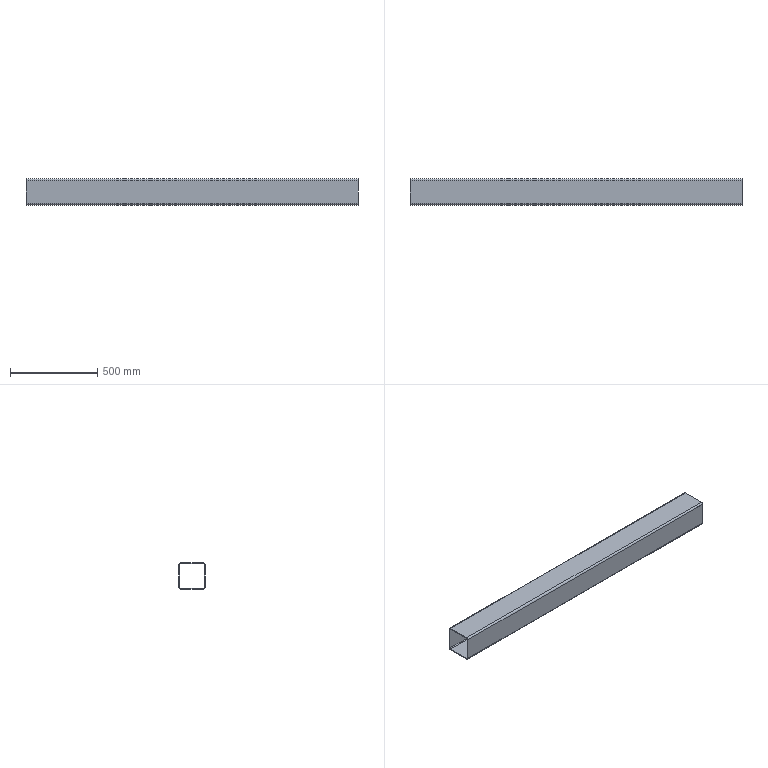Part | SolidWorks | features WeldMemberFeat 1, WeldmentFeature 1 | 1 solid | 18 faces | box 1900 x 150 x 150 mm | volume 5387677 mm3 | plane 10 | cylinder 8 | commonest cylinder face diameters 10 x4 20 x4
STEP:
#1=CARTESIAN_POINT('',(-950.,75.,65.));
#2=VERTEX_POINT('',#1);
#3=CARTESIAN_POINT('',(-950.,65.,75.));
#4=VERTEX_POINT('',#3);
#5=CARTESIAN_POINT('',(-950.,65.,65.));
#6=DIRECTION('',(1.,0.,0.));
#7=DIRECTION('',(0.,1.,0.));
#8=AXIS2_PLACEMENT_3D('',#5,#6,#7);
#9=CIRCLE('',#8,10.);
#10=EDGE_CURVE('',#2,#4,#9,.T.);
#11=ORIENTED_EDGE('',*,*,#10,.T.);
#12=CARTESIAN_POINT('',(950.,65.,75.));
#13=VERTEX_POINT('',#12);
#14=CARTESIAN_POINT('',(950.,65.,75.));
#15=DIRECTION('',(-1.,0.,0.));
#16=VECTOR('',#15,1000.);
#17=LINE('',#14,#16);
#18=EDGE_CURVE('',#13,#4,#17,.T.);
#19=ORIENTED_EDGE('',*,*,#18,.F.);
#20=CARTESIAN_POINT('',(950.,75.,65.));
#21=VERTEX_POINT('',#20);
#22=CARTESIAN_POINT('',(950.,65.,65.));
#23=DIRECTION('',(1.,0.,0.));
#24=DIRECTION('',(0.,1.,0.));
#25=AXIS2_PLACEMENT_3D('',#22,#23,#24);
#26=CIRCLE('',#25,10.);
#27=EDGE_CURVE('',#21,#13,#26,.T.);
#28=ORIENTED_EDGE('',*,*,#27,.F.);
#29=CARTESIAN_POINT('',(950.,75.,65.));
#30=DIRECTION('',(-1.,0.,0.));
#31=VECTOR('',#30,1000.);
#32=LINE('',#29,#31);
#33=EDGE_CURVE('',#21,#2,#32,.T.);
#34=ORIENTED_EDGE('',*,*,#33,.T.);
#35=EDGE_LOOP('',(#11,#19,#28,#34));
#36=FACE_OUTER_BOUND('',#35,.T.);
#37=CARTESIAN_POINT('',(950.,65.,65.));
#38=DIRECTION('',(-1.,0.,0.));
#39=DIRECTION('',(0.,-1.,0.));
#40=AXIS2_PLACEMENT_3D('',#37,#38,#39);
#41=CYLINDRICAL_SURFACE('',#40,10.);
#42=ADVANCED_FACE('',(#36),#41,.T.);
#43=CARTESIAN_POINT('',(-950.,-65.,75.));
#44=VERTEX_POINT('',#43);
#45=CARTESIAN_POINT('',(-950.,65.,75.));
#46=DIRECTION('',(0.,-1.,0.));
#47=VECTOR('',#46,1000.);
#48=LINE('',#45,#47);
#49=EDGE_CURVE('',#4,#44,#48,.T.);
#50=ORIENTED_EDGE('',*,*,#49,.T.);
#51=CARTESIAN_POINT('',(950.,-65.,75.));
#52=VERTEX_POINT('',#51);
#53=CARTESIAN_POINT('',(950.,-65.,75.));
#54=DIRECTION('',(-1.,0.,0.));
#55=VECTOR('',#54,1000.);
#56=LINE('',#53,#55);
#57=EDGE_CURVE('',#52,#44,#56,.T.);
#58=ORIENTED_EDGE('',*,*,#57,.F.);
#59=CARTESIAN_POINT('',(950.,65.,75.));
#60=DIRECTION('',(0.,-1.,0.));
#61=VECTOR('',#60,1000.);
#62=LINE('',#59,#61);
#63=EDGE_CURVE('',#13,#52,#62,.T.);
#64=ORIENTED_EDGE('',*,*,#63,.F.);
#65=ORIENTED_EDGE('',*,*,#18,.T.);
#66=EDGE_LOOP('',(#50,#58,#64,#65));
#67=FACE_OUTER_BOUND('',#66,.T.);
#68=CARTESIAN_POINT('',(950.,65.,75.));
#69=DIRECTION('',(0.,0.,-1.));
#70=DIRECTION('',(-1.,0.,0.));
#71=AXIS2_PLACEMENT_3D('',#68,#69,#70);
#72=PLANE('',#71);
#73=ADVANCED_FACE('',(#67),#72,.F.);
#74=CARTESIAN_POINT('',(-950.,-75.,65.));
#75=VERTEX_POINT('',#74);
#76=CARTESIAN_POINT('',(-950.,-65.,65.));
#77=DIRECTION('',(1.,0.,0.));
#78=DIRECTION('',(0.,1.,0.));
#79=AXIS2_PLACEMENT_3D('',#76,#77,#78);
#80=CIRCLE('',#79,10.);
#81=EDGE_CURVE('',#44,#75,#80,.T.);
#82=ORIENTED_EDGE('',*,*,#81,.T.);
#83=CARTESIAN_POINT('',(950.,-75.,65.));
#84=VERTEX_POINT('',#83);
#85=CARTESIAN_POINT('',(950.,-75.,65.));
#86=DIRECTION('',(-1.,0.,0.));
#87=VECTOR('',#86,1000.);
#88=LINE('',#85,#87);
#89=EDGE_CURVE('',#84,#75,#88,.T.);
#90=ORIENTED_EDGE('',*,*,#89,.F.);
#91=CARTESIAN_POINT('',(950.,-65.,65.));
#92=DIRECTION('',(1.,0.,0.));
#93=DIRECTION('',(0.,1.,0.));
#94=AXIS2_PLACEMENT_3D('',#91,#92,#93);
#95=CIRCLE('',#94,10.);
#96=EDGE_CURVE('',#52,#84,#95,.T.);
#97=ORIENTED_EDGE('',*,*,#96,.F.);
#98=ORIENTED_EDGE('',*,*,#57,.T.);
#99=EDGE_LOOP('',(#82,#90,#97,#98));
#100=FACE_OUTER_BOUND('',#99,.T.);
#101=CARTESIAN_POINT('',(950.,-65.,65.));
#102=DIRECTION('',(-1.,0.,0.));
#103=DIRECTION('',(0.,-1.,0.));
#104=AXIS2_PLACEMENT_3D('',#101,#102,#103);
#105=CYLINDRICAL_SURFACE('',#104,10.);
#106=ADVANCED_FACE('',(#100),#105,.T.);
#107=CARTESIAN_POINT('',(-950.,-75.,-65.));
#108=VERTEX_POINT('',#107);
#109=CARTESIAN_POINT('',(-950.,-75.,-65.));
#110=DIRECTION('',(0.,0.,-1.));
#111=VECTOR('',#110,1000.);
#112=LINE('',#109,#111);
#113=EDGE_CURVE('',#75,#108,#112,.T.);
#114=ORIENTED_EDGE('',*,*,#113,.T.);
#115=CARTESIAN_POINT('',(950.,-75.,-65.));
#116=VERTEX_POINT('',#115);
#117=CARTESIAN_POINT('',(950.,-75.,-65.));
#118=DIRECTION('',(-1.,0.,0.));
#119=VECTOR('',#118,1000.);
#120=LINE('',#117,#119);
#121=EDGE_CURVE('',#116,#108,#120,.T.);
#122=ORIENTED_EDGE('',*,*,#121,.F.);
#123=CARTESIAN_POINT('',(950.,-75.,-65.));
#124=DIRECTION('',(0.,0.,-1.));
#125=VECTOR('',#124,1000.);
#126=LINE('',#123,#125);
#127=EDGE_CURVE('',#84,#116,#126,.T.);
#128=ORIENTED_EDGE('',*,*,#127,.F.);
#129=ORIENTED_EDGE('',*,*,#89,.T.);
#130=EDGE_LOOP('',(#114,#122,#128,#129));
#131=FACE_OUTER_BOUND('',#130,.T.);
#132=CARTESIAN_POINT('',(950.,-75.,-65.));
#133=DIRECTION('',(0.,1.,0.));
#134=DIRECTION('',(-1.,0.,0.));
#135=AXIS2_PLACEMENT_3D('',#132,#133,#134);
#136=PLANE('',#135);
#137=ADVANCED_FACE('',(#131),#136,.F.);
#138=CARTESIAN_POINT('',(-950.,-65.,-75.));
#139=VERTEX_POINT('',#138);
#140=CARTESIAN_POINT('',(-950.,-65.,-65.));
#141=DIRECTION('',(1.,0.,0.));
#142=DIRECTION('',(0.,1.,0.));
#143=AXIS2_PLACEMENT_3D('',#140,#141,#142);
#144=CIRCLE('',#143,10.);
#145=EDGE_CURVE('',#108,#139,#144,.T.);
#146=ORIENTED_EDGE('',*,*,#145,.T.);
#147=CARTESIAN_POINT('',(950.,-65.,-75.));
#148=VERTEX_POINT('',#147);
#149=CARTESIAN_POINT('',(950.,-65.,-75.));
#150=DIRECTION('',(-1.,0.,0.));
#151=VECTOR('',#150,1000.);
#152=LINE('',#149,#151);
#153=EDGE_CURVE('',#148,#139,#152,.T.);
#154=ORIENTED_EDGE('',*,*,#153,.F.);
#155=CARTESIAN_POINT('',(950.,-65.,-65.));
#156=DIRECTION('',(1.,0.,0.));
#157=DIRECTION('',(0.,1.,0.));
#158=AXIS2_PLACEMENT_3D('',#155,#156,#157);
#159=CIRCLE('',#158,10.);
#160=EDGE_CURVE('',#116,#148,#159,.T.);
#161=ORIENTED_EDGE('',*,*,#160,.F.);
#162=ORIENTED_EDGE('',*,*,#121,.T.);
#163=EDGE_LOOP('',(#146,#154,#161,#162));
#164=FACE_OUTER_BOUND('',#163,.T.);
#165=CARTESIAN_POINT('',(950.,-65.,-65.));
#166=DIRECTION('',(-1.,0.,0.));
#167=DIRECTION('',(0.,-1.,0.));
#168=AXIS2_PLACEMENT_3D('',#165,#166,#167);
#169=CYLINDRICAL_SURFACE('',#168,10.);
#170=ADVANCED_FACE('',(#164),#169,.T.);
#171=CARTESIAN_POINT('',(-950.,65.,-75.));
#172=VERTEX_POINT('',#171);
#173=CARTESIAN_POINT('',(-950.,-65.,-75.));
#174=DIRECTION('',(0.,1.,0.));
#175=VECTOR('',#174,1000.);
#176=LINE('',#173,#175);
#177=EDGE_CURVE('',#139,#172,#176,.T.);
#178=ORIENTED_EDGE('',*,*,#177,.T.);
#179=CARTESIAN_POINT('',(950.,65.,-75.));
#180=VERTEX_POINT('',#179);
#181=CARTESIAN_POINT('',(950.,65.,-75.));
#182=DIRECTION('',(-1.,0.,0.));
#183=VECTOR('',#182,1000.);
#184=LINE('',#181,#183);
#185=EDGE_CURVE('',#180,#172,#184,.T.);
#186=ORIENTED_EDGE('',*,*,#185,.F.);
#187=CARTESIAN_POINT('',(950.,-65.,-75.));
#188=DIRECTION('',(0.,1.,0.));
#189=VECTOR('',#188,1000.);
#190=LINE('',#187,#189);
#191=EDGE_CURVE('',#148,#180,#190,.T.);
#192=ORIENTED_EDGE('',*,*,#191,.F.);
#193=ORIENTED_EDGE('',*,*,#153,.T.);
#194=EDGE_LOOP('',(#178,#186,#192,#193));
#195=FACE_OUTER_BOUND('',#194,.T.);
#196=CARTESIAN_POINT('',(950.,-65.,-75.));
#197=DIRECTION('',(0.,0.,1.));
#198=DIRECTION('',(1.,0.,0.));
#199=AXIS2_PLACEMENT_3D('',#196,#197,#198);
#200=PLANE('',#199);
#201=ADVANCED_FACE('',(#195),#200,.F.);
#202=CARTESIAN_POINT('',(-950.,75.,-65.));
#203=VERTEX_POINT('',#202);
#204=CARTESIAN_POINT('',(-950.,65.,-65.));
#205=DIRECTION('',(1.,0.,0.));
#206=DIRECTION('',(0.,1.,0.));
#207=AXIS2_PLACEMENT_3D('',#204,#205,#206);
#208=CIRCLE('',#207,10.);
#209=EDGE_CURVE('',#172,#203,#208,.T.);
#210=ORIENTED_EDGE('',*,*,#209,.T.);
#211=CARTESIAN_POINT('',(950.,75.,-65.));
#212=VERTEX_POINT('',#211);
#213=CARTESIAN_POINT('',(950.,75.,-65.));
#214=DIRECTION('',(-1.,0.,0.));
#215=VECTOR('',#214,1000.);
#216=LINE('',#213,#215);
#217=EDGE_CURVE('',#212,#203,#216,.T.);
#218=ORIENTED_EDGE('',*,*,#217,.F.);
#219=CARTESIAN_POINT('',(950.,65.,-65.));
#220=DIRECTION('',(1.,0.,0.));
#221=DIRECTION('',(0.,1.,0.));
#222=AXIS2_PLACEMENT_3D('',#219,#220,#221);
#223=CIRCLE('',#222,10.);
#224=EDGE_CURVE('',#180,#212,#223,.T.);
#225=ORIENTED_EDGE('',*,*,#224,.F.);
#226=ORIENTED_EDGE('',*,*,#185,.T.);
#227=EDGE_LOOP('',(#210,#218,#225,#226));
#228=FACE_OUTER_BOUND('',#227,.T.);
#229=CARTESIAN_POINT('',(950.,65.,-65.));
#230=DIRECTION('',(-1.,0.,0.));
#231=DIRECTION('',(0.,-1.,0.));
#232=AXIS2_PLACEMENT_3D('',#229,#230,#231);
#233=CYLINDRICAL_SURFACE('',#232,10.);
#234=ADVANCED_FACE('',(#228),#233,.T.);
#235=CARTESIAN_POINT('',(-950.,-65.,70.));
#236=VERTEX_POINT('',#235);
#237=CARTESIAN_POINT('',(-950.,-70.,65.));
#238=VERTEX_POINT('',#237);
#239=CARTESIAN_POINT('',(-950.,-65.,65.));
#240=DIRECTION('',(1.,0.,0.));
#241=DIRECTION('',(0.,1.,0.));
#242=AXIS2_PLACEMENT_3D('',#239,#240,#241);
#243=CIRCLE('',#242,5.);
#244=EDGE_CURVE('',#236,#238,#243,.T.);
#245=ORIENTED_EDGE('',*,*,#244,.F.);
#246=CARTESIAN_POINT('',(950.,-65.,70.));
#247=VERTEX_POINT('',#246);
#248=CARTESIAN_POINT('',(950.,-65.,70.));
#249=DIRECTION('',(-1.,0.,0.));
#250=VECTOR('',#249,1000.);
#251=LINE('',#248,#250);
#252=EDGE_CURVE('',#247,#236,#251,.T.);
#253=ORIENTED_EDGE('',*,*,#252,.F.);
#254=CARTESIAN_POINT('',(950.,-70.,65.));
#255=VERTEX_POINT('',#254);
#256=CARTESIAN_POINT('',(950.,-65.,65.));
#257=DIRECTION('',(1.,0.,0.));
#258=DIRECTION('',(0.,1.,0.));
#259=AXIS2_PLACEMENT_3D('',#256,#257,#258);
#260=CIRCLE('',#259,5.);
#261=EDGE_CURVE('',#247,#255,#260,.T.);
#262=ORIENTED_EDGE('',*,*,#261,.T.);
#263=CARTESIAN_POINT('',(950.,-70.,65.));
#264=DIRECTION('',(-1.,0.,0.));
#265=VECTOR('',#264,1000.);
#266=LINE('',#263,#265);
#267=EDGE_CURVE('',#255,#238,#266,.T.);
#268=ORIENTED_EDGE('',*,*,#267,.T.);
#269=EDGE_LOOP('',(#245,#253,#262,#268));
#270=FACE_OUTER_BOUND('',#269,.T.);
#271=CARTESIAN_POINT('',(950.,-65.,65.));
#272=DIRECTION('',(-1.,0.,0.));
#273=DIRECTION('',(0.,-1.,0.));
#274=AXIS2_PLACEMENT_3D('',#271,#272,#273);
#275=CYLINDRICAL_SURFACE('',#274,5.);
#276=ADVANCED_FACE('',(#270),#275,.F.);
#277=CARTESIAN_POINT('',(-950.,65.,70.));
#278=VERTEX_POINT('',#277);
#279=CARTESIAN_POINT('',(-950.,65.,70.));
#280=DIRECTION('',(0.,-1.,0.));
#281=VECTOR('',#280,1000.);
#282=LINE('',#279,#281);
#283=EDGE_CURVE('',#278,#236,#282,.T.);
#284=ORIENTED_EDGE('',*,*,#283,.F.);
#285=CARTESIAN_POINT('',(950.,65.,70.));
#286=VERTEX_POINT('',#285);
#287=CARTESIAN_POINT('',(950.,65.,70.));
#288=DIRECTION('',(-1.,0.,0.));
#289=VECTOR('',#288,1000.);
#290=LINE('',#287,#289);
#291=EDGE_CURVE('',#286,#278,#290,.T.);
#292=ORIENTED_EDGE('',*,*,#291,.F.);
#293=CARTESIAN_POINT('',(950.,65.,70.));
#294=DIRECTION('',(0.,-1.,0.));
#295=VECTOR('',#294,1000.);
#296=LINE('',#293,#295);
#297=EDGE_CURVE('',#286,#247,#296,.T.);
#298=ORIENTED_EDGE('',*,*,#297,.T.);
#299=ORIENTED_EDGE('',*,*,#252,.T.);
#300=EDGE_LOOP('',(#284,#292,#298,#299));
#301=FACE_OUTER_BOUND('',#300,.T.);
#302=CARTESIAN_POINT('',(950.,65.,70.));
#303=DIRECTION('',(0.,0.,-1.));
#304=DIRECTION('',(-1.,0.,0.));
#305=AXIS2_PLACEMENT_3D('',#302,#303,#304);
#306=PLANE('',#305);
#307=ADVANCED_FACE('',(#301),#306,.T.);
#308=CARTESIAN_POINT('',(-950.,70.,65.));
#309=VERTEX_POINT('',#308);
#310=CARTESIAN_POINT('',(-950.,65.,65.));
#311=DIRECTION('',(1.,0.,0.));
#312=DIRECTION('',(0.,1.,0.));
#313=AXIS2_PLACEMENT_3D('',#310,#311,#312);
#314=CIRCLE('',#313,5.);
#315=EDGE_CURVE('',#309,#278,#314,.T.);
#316=ORIENTED_EDGE('',*,*,#315,.F.);
#317=CARTESIAN_POINT('',(950.,70.,65.));
#318=VERTEX_POINT('',#317);
#319=CARTESIAN_POINT('',(950.,70.,65.));
#320=DIRECTION('',(-1.,0.,0.));
#321=VECTOR('',#320,1000.);
#322=LINE('',#319,#321);
#323=EDGE_CURVE('',#318,#309,#322,.T.);
#324=ORIENTED_EDGE('',*,*,#323,.F.);
#325=CARTESIAN_POINT('',(950.,65.,65.));
#326=DIRECTION('',(1.,0.,0.));
#327=DIRECTION('',(0.,1.,0.));
#328=AXIS2_PLACEMENT_3D('',#325,#326,#327);
#329=CIRCLE('',#328,5.);
#330=EDGE_CURVE('',#318,#286,#329,.T.);
#331=ORIENTED_EDGE('',*,*,#330,.T.);
#332=ORIENTED_EDGE('',*,*,#291,.T.);
#333=EDGE_LOOP('',(#316,#324,#331,#332));
#334=FACE_OUTER_BOUND('',#333,.T.);
#335=CARTESIAN_POINT('',(950.,65.,65.));
#336=DIRECTION('',(-1.,0.,0.));
#337=DIRECTION('',(0.,-1.,0.));
#338=AXIS2_PLACEMENT_3D('',#335,#336,#337);
#339=CYLINDRICAL_SURFACE('',#338,5.);
#340=ADVANCED_FACE('',(#334),#339,.F.);
#341=CARTESIAN_POINT('',(-950.,70.,-65.));
#342=VERTEX_POINT('',#341);
#343=CARTESIAN_POINT('',(-950.,70.,65.));
#344=DIRECTION('',(0.,0.,1.));
#345=VECTOR('',#344,1000.);
#346=LINE('',#343,#345);
#347=EDGE_CURVE('',#342,#309,#346,.T.);
#348=ORIENTED_EDGE('',*,*,#347,.F.);
#349=CARTESIAN_POINT('',(950.,70.,-65.));
#350=VERTEX_POINT('',#349);
#351=CARTESIAN_POINT('',(950.,70.,-65.));
#352=DIRECTION('',(-1.,0.,0.));
#353=VECTOR('',#352,1000.);
#354=LINE('',#351,#353);
#355=EDGE_CURVE('',#350,#342,#354,.T.);
#356=ORIENTED_EDGE('',*,*,#355,.F.);
#357=CARTESIAN_POINT('',(950.,70.,65.));
#358=DIRECTION('',(0.,0.,1.));
#359=VECTOR('',#358,1000.);
#360=LINE('',#357,#359);
#361=EDGE_CURVE('',#350,#318,#360,.T.);
#362=ORIENTED_EDGE('',*,*,#361,.T.);
#363=ORIENTED_EDGE('',*,*,#323,.T.);
#364=EDGE_LOOP('',(#348,#356,#362,#363));
#365=FACE_OUTER_BOUND('',#364,.T.);
#366=CARTESIAN_POINT('',(950.,70.,65.));
#367=DIRECTION('',(0.,-1.,0.));
#368=DIRECTION('',(1.,0.,0.));
#369=AXIS2_PLACEMENT_3D('',#366,#367,#368);
#370=PLANE('',#369);
#371=ADVANCED_FACE('',(#365),#370,.T.);
#372=CARTESIAN_POINT('',(-950.,65.,-70.));
#373=VERTEX_POINT('',#372);
#374=CARTESIAN_POINT('',(-950.,65.,-65.));
#375=DIRECTION('',(1.,0.,0.));
#376=DIRECTION('',(0.,1.,0.));
#377=AXIS2_PLACEMENT_3D('',#374,#375,#376);
#378=CIRCLE('',#377,5.);
#379=EDGE_CURVE('',#373,#342,#378,.T.);
#380=ORIENTED_EDGE('',*,*,#379,.F.);
#381=CARTESIAN_POINT('',(950.,65.,-70.));
#382=VERTEX_POINT('',#381);
#383=CARTESIAN_POINT('',(950.,65.,-70.));
#384=DIRECTION('',(-1.,0.,0.));
#385=VECTOR('',#384,1000.);
#386=LINE('',#383,#385);
#387=EDGE_CURVE('',#382,#373,#386,.T.);
#388=ORIENTED_EDGE('',*,*,#387,.F.);
#389=CARTESIAN_POINT('',(950.,65.,-65.));
#390=DIRECTION('',(1.,0.,0.));
#391=DIRECTION('',(0.,1.,0.));
#392=AXIS2_PLACEMENT_3D('',#389,#390,#391);
#393=CIRCLE('',#392,5.);
#394=EDGE_CURVE('',#382,#350,#393,.T.);
#395=ORIENTED_EDGE('',*,*,#394,.T.);
#396=ORIENTED_EDGE('',*,*,#355,.T.);
#397=EDGE_LOOP('',(#380,#388,#395,#396));
#398=FACE_OUTER_BOUND('',#397,.T.);
#399=CARTESIAN_POINT('',(950.,65.,-65.));
#400=DIRECTION('',(-1.,0.,0.));
#401=DIRECTION('',(0.,-1.,0.));
#402=AXIS2_PLACEMENT_3D('',#399,#400,#401);
#403=CYLINDRICAL_SURFACE('',#402,5.);
#404=ADVANCED_FACE('',(#398),#403,.F.);
#405=CARTESIAN_POINT('',(-950.,-65.,-70.));
#406=VERTEX_POINT('',#405);
#407=CARTESIAN_POINT('',(-950.,-65.,-70.));
#408=DIRECTION('',(0.,1.,0.));
#409=VECTOR('',#408,1000.);
#410=LINE('',#407,#409);
#411=EDGE_CURVE('',#406,#373,#410,.T.);
#412=ORIENTED_EDGE('',*,*,#411,.F.);
#413=CARTESIAN_POINT('',(950.,-65.,-70.));
#414=VERTEX_POINT('',#413);
#415=CARTESIAN_POINT('',(950.,-65.,-70.));
#416=DIRECTION('',(-1.,0.,0.));
#417=VECTOR('',#416,1000.);
#418=LINE('',#415,#417);
#419=EDGE_CURVE('',#414,#406,#418,.T.);
#420=ORIENTED_EDGE('',*,*,#419,.F.);
#421=CARTESIAN_POINT('',(950.,-65.,-70.));
#422=DIRECTION('',(0.,1.,0.));
#423=VECTOR('',#422,1000.);
#424=LINE('',#421,#423);
#425=EDGE_CURVE('',#414,#382,#424,.T.);
#426=ORIENTED_EDGE('',*,*,#425,.T.);
#427=ORIENTED_EDGE('',*,*,#387,.T.);
#428=EDGE_LOOP('',(#412,#420,#426,#427));
#429=FACE_OUTER_BOUND('',#428,.T.);
#430=CARTESIAN_POINT('',(950.,-65.,-70.));
#431=DIRECTION('',(0.,0.,1.));
#432=DIRECTION('',(1.,0.,0.));
#433=AXIS2_PLACEMENT_3D('',#430,#431,#432);
#434=PLANE('',#433);
#435=ADVANCED_FACE('',(#429),#434,.T.);
#436=CARTESIAN_POINT('',(-950.,-70.,-65.));
#437=VERTEX_POINT('',#436);
#438=CARTESIAN_POINT('',(-950.,-65.,-65.));
#439=DIRECTION('',(1.,0.,0.));
#440=DIRECTION('',(0.,1.,0.));
#441=AXIS2_PLACEMENT_3D('',#438,#439,#440);
#442=CIRCLE('',#441,5.);
#443=EDGE_CURVE('',#437,#406,#442,.T.);
#444=ORIENTED_EDGE('',*,*,#443,.F.);
#445=CARTESIAN_POINT('',(950.,-70.,-65.));
#446=VERTEX_POINT('',#445);
#447=CARTESIAN_POINT('',(950.,-70.,-65.));
#448=DIRECTION('',(-1.,0.,0.));
#449=VECTOR('',#448,1000.);
#450=LINE('',#447,#449);
#451=EDGE_CURVE('',#446,#437,#450,.T.);
#452=ORIENTED_EDGE('',*,*,#451,.F.);
#453=CARTESIAN_POINT('',(950.,-65.,-65.));
#454=DIRECTION('',(1.,0.,0.));
#455=DIRECTION('',(0.,1.,0.));
#456=AXIS2_PLACEMENT_3D('',#453,#454,#455);
#457=CIRCLE('',#456,5.);
#458=EDGE_CURVE('',#446,#414,#457,.T.);
#459=ORIENTED_EDGE('',*,*,#458,.T.);
#460=ORIENTED_EDGE('',*,*,#419,.T.);
#461=EDGE_LOOP('',(#444,#452,#459,#460));
#462=FACE_OUTER_BOUND('',#461,.T.);
#463=CARTESIAN_POINT('',(950.,-65.,-65.));
#464=DIRECTION('',(-1.,0.,0.));
#465=DIRECTION('',(0.,-1.,0.));
#466=AXIS2_PLACEMENT_3D('',#463,#464,#465);
#467=CYLINDRICAL_SURFACE('',#466,5.);
#468=ADVANCED_FACE('',(#462),#467,.F.);
#469=CARTESIAN_POINT('',(-950.,-70.,-65.));
#470=DIRECTION('',(0.,0.,-1.));
#471=VECTOR('',#470,1000.);
#472=LINE('',#469,#471);
#473=EDGE_CURVE('',#238,#437,#472,.T.);
#474=ORIENTED_EDGE('',*,*,#473,.F.);
#475=ORIENTED_EDGE('',*,*,#267,.F.);
#476=CARTESIAN_POINT('',(950.,-70.,-65.));
#477=DIRECTION('',(0.,0.,-1.));
#478=VECTOR('',#477,1000.);
#479=LINE('',#476,#478);
#480=EDGE_CURVE('',#255,#446,#479,.T.);
#481=ORIENTED_EDGE('',*,*,#480,.T.);
#482=ORIENTED_EDGE('',*,*,#451,.T.);
#483=EDGE_LOOP('',(#474,#475,#481,#482));
#484=FACE_OUTER_BOUND('',#483,.T.);
#485=CARTESIAN_POINT('',(950.,-70.,-65.));
#486=DIRECTION('',(0.,1.,0.));
#487=DIRECTION('',(-1.,0.,0.));
#488=AXIS2_PLACEMENT_3D('',#485,#486,#487);
#489=PLANE('',#488);
#490=ADVANCED_FACE('',(#484),#489,.T.);
#491=CARTESIAN_POINT('',(-950.,75.,65.));
#492=DIRECTION('',(0.,0.,1.));
#493=VECTOR('',#492,1000.);
#494=LINE('',#491,#493);
#495=EDGE_CURVE('',#203,#2,#494,.T.);
#496=ORIENTED_EDGE('',*,*,#495,.T.);
#497=ORIENTED_EDGE('',*,*,#33,.F.);
#498=CARTESIAN_POINT('',(950.,75.,65.));
#499=DIRECTION('',(0.,0.,1.));
#500=VECTOR('',#499,1000.);
#501=LINE('',#498,#500);
#502=EDGE_CURVE('',#212,#21,#501,.T.);
#503=ORIENTED_EDGE('',*,*,#502,.F.);
#504=ORIENTED_EDGE('',*,*,#217,.T.);
#505=EDGE_LOOP('',(#496,#497,#503,#504));
#506=FACE_OUTER_BOUND('',#505,.T.);
#507=CARTESIAN_POINT('',(950.,75.,65.));
#508=DIRECTION('',(0.,-1.,0.));
#509=DIRECTION('',(1.,0.,0.));
#510=AXIS2_PLACEMENT_3D('',#507,#508,#509);
#511=PLANE('',#510);
#512=ADVANCED_FACE('',(#506),#511,.F.);
#513=ORIENTED_EDGE('',*,*,#261,.F.);
#514=ORIENTED_EDGE('',*,*,#297,.F.);
#515=ORIENTED_EDGE('',*,*,#330,.F.);
#516=ORIENTED_EDGE('',*,*,#361,.F.);
#517=ORIENTED_EDGE('',*,*,#394,.F.);
#518=ORIENTED_EDGE('',*,*,#425,.F.);
#519=ORIENTED_EDGE('',*,*,#458,.F.);
#520=ORIENTED_EDGE('',*,*,#480,.F.);
#521=EDGE_LOOP('',(#513,#514,#515,#516,#517,#518,#519,#520));
#522=FACE_BOUND('',#521,.T.);
#523=ORIENTED_EDGE('',*,*,#27,.T.);
#524=ORIENTED_EDGE('',*,*,#63,.T.);
#525=ORIENTED_EDGE('',*,*,#96,.T.);
#526=ORIENTED_EDGE('',*,*,#127,.T.);
#527=ORIENTED_EDGE('',*,*,#160,.T.);
#528=ORIENTED_EDGE('',*,*,#191,.T.);
#529=ORIENTED_EDGE('',*,*,#224,.T.);
#530=ORIENTED_EDGE('',*,*,#502,.T.);
#531=EDGE_LOOP('',(#523,#524,#525,#526,#527,#528,#529,#530));
#532=FACE_OUTER_BOUND('',#531,.T.);
#533=CARTESIAN_POINT('',(950.,65.,65.));
#534=DIRECTION('',(1.,0.,0.));
#535=DIRECTION('',(0.,1.,0.));
#536=AXIS2_PLACEMENT_3D('',#533,#534,#535);
#537=PLANE('',#536);
#538=ADVANCED_FACE('',(#522,#532),#537,.T.);
#539=ORIENTED_EDGE('',*,*,#244,.T.);
#540=ORIENTED_EDGE('',*,*,#473,.T.);
#541=ORIENTED_EDGE('',*,*,#443,.T.);
#542=ORIENTED_EDGE('',*,*,#411,.T.);
#543=ORIENTED_EDGE('',*,*,#379,.T.);
#544=ORIENTED_EDGE('',*,*,#347,.T.);
#545=ORIENTED_EDGE('',*,*,#315,.T.);
#546=ORIENTED_EDGE('',*,*,#283,.T.);
#547=EDGE_LOOP('',(#539,#540,#541,#542,#543,#544,#545,#546));
#548=FACE_BOUND('',#547,.T.);
#549=ORIENTED_EDGE('',*,*,#10,.F.);
#550=ORIENTED_EDGE('',*,*,#495,.F.);
#551=ORIENTED_EDGE('',*,*,#209,.F.);
#552=ORIENTED_EDGE('',*,*,#177,.F.);
#553=ORIENTED_EDGE('',*,*,#145,.F.);
#554=ORIENTED_EDGE('',*,*,#113,.F.);
#555=ORIENTED_EDGE('',*,*,#81,.F.);
#556=ORIENTED_EDGE('',*,*,#49,.F.);
#557=EDGE_LOOP('',(#549,#550,#551,#552,#553,#554,#555,#556));
#558=FACE_OUTER_BOUND('',#557,.T.);
#559=CARTESIAN_POINT('',(-950.,65.,65.));
#560=DIRECTION('',(1.,0.,0.));
#561=DIRECTION('',(0.,1.,0.));
#562=AXIS2_PLACEMENT_3D('',#559,#560,#561);
#563=PLANE('',#562);
#564=ADVANCED_FACE('',(#548,#558),#563,.F.);
#565=CLOSED_SHELL('',(#42,#73,#106,#137,#170,#201,#234,#276,#307,#340,#371,#404,#435,#468,#490,#512,#538,#564));
#566=MANIFOLD_SOLID_BREP('',#565);
#567=CARTESIAN_POINT('',(0.,0.,0.));
#568=DIRECTION('',(0.,0.,1.));
#569=DIRECTION('',(1.,0.,0.));
#570=AXIS2_PLACEMENT_3D('',#567,#568,#569);
#571=(LENGTH_UNIT()NAMED_UNIT(*)SI_UNIT(.MILLI.,.METRE.));
#572=UNCERTAINTY_MEASURE_WITH_UNIT(LENGTH_MEASURE(0.00001),#571,'','');
#573=(NAMED_UNIT(*)PLANE_ANGLE_UNIT()SI_UNIT($,.RADIAN.));
#574=(NAMED_UNIT(*)SI_UNIT($,.STERADIAN.)SOLID_ANGLE_UNIT());
#575=(GEOMETRIC_REPRESENTATION_CONTEXT(3)GLOBAL_UNCERTAINTY_ASSIGNED_CONTEXT((#572))GLOBAL_UNIT_ASSIGNED_CONTEXT((#571,#573,#574))REPRESENTATION_CONTEXT('',''));
#576=ADVANCED_BREP_SHAPE_REPRESENTATION('',(#566,#570),#575);